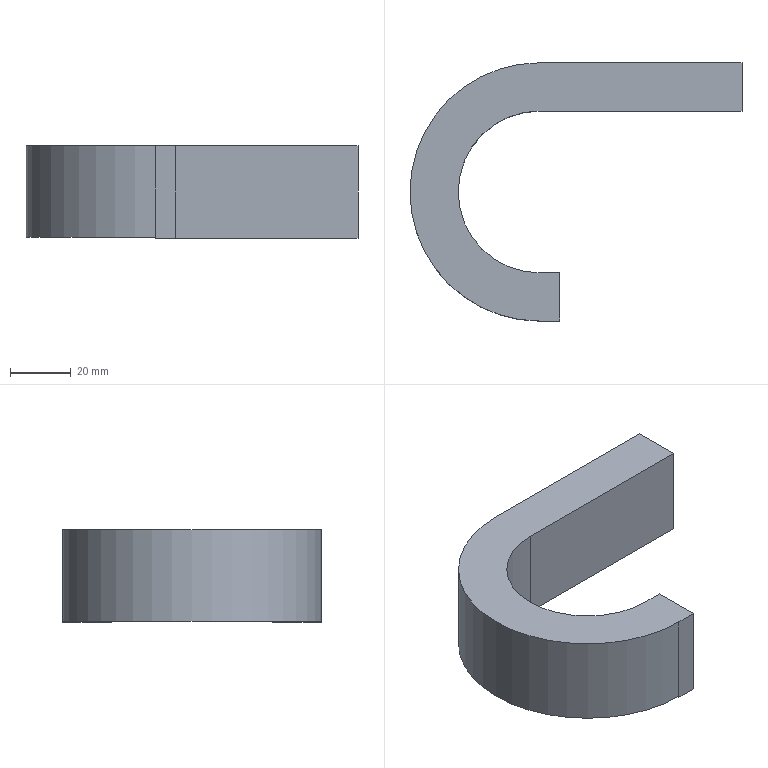Part | STEP file | RS40-AS-2LSR-T-266L-JR-Part-181 | 1 solid | 14 faces | box 109.3 x 85 x 30.35 mm | volume 87244 mm3 | plane 12 | cylinder 2 | commonest cylinder face diameters 53.238 x1 85 x1
STEP:
#1=CARTESIAN_POINT('',(1463.84,85.,30.35));
#2=VERTEX_POINT('',#1);
#3=CARTESIAN_POINT('',(1530.64,85.,30.35));
#4=VERTEX_POINT('',#3);
#5=CARTESIAN_POINT('',(1497.24,85.,30.35));
#6=DIRECTION('',(1.,0.,0.));
#7=VECTOR('',#6,1000.);
#8=LINE('',#5,#7);
#9=EDGE_CURVE('',#2,#4,#8,.T.);
#10=ORIENTED_EDGE('',*,*,#9,.F.);
#11=CARTESIAN_POINT('',(1463.84,0.00006,30.35));
#12=VERTEX_POINT('',#11);
#13=CARTESIAN_POINT('',(1463.84,42.5,30.35));
#14=DIRECTION('',(0.,0.,-1.));
#15=DIRECTION('',(0.,1.,0.));
#16=AXIS2_PLACEMENT_3D('',#13,#14,#15);
#17=CIRCLE('',#16,42.5);
#18=EDGE_CURVE('',#12,#2,#17,.T.);
#19=ORIENTED_EDGE('',*,*,#18,.F.);
#20=CARTESIAN_POINT('',(1470.64,0.00006,30.35));
#21=VERTEX_POINT('',#20);
#22=CARTESIAN_POINT('',(1467.24,0.00006,30.35));
#23=DIRECTION('',(-1.,0.,0.));
#24=VECTOR('',#23,1000.);
#25=LINE('',#22,#24);
#26=EDGE_CURVE('',#21,#12,#25,.T.);
#27=ORIENTED_EDGE('',*,*,#26,.F.);
#28=CARTESIAN_POINT('',(1470.64,15.881,30.35));
#29=VERTEX_POINT('',#28);
#30=CARTESIAN_POINT('',(1470.64,7.941,30.35));
#31=DIRECTION('',(0.,-1.,0.));
#32=VECTOR('',#31,1000.);
#33=LINE('',#30,#32);
#34=EDGE_CURVE('',#29,#21,#33,.T.);
#35=ORIENTED_EDGE('',*,*,#34,.F.);
#36=CARTESIAN_POINT('',(1463.84,15.881,30.35));
#37=VERTEX_POINT('',#36);
#38=CARTESIAN_POINT('',(1467.24,15.881,30.35));
#39=DIRECTION('',(1.,0.,0.));
#40=VECTOR('',#39,1000.);
#41=LINE('',#38,#40);
#42=EDGE_CURVE('',#37,#29,#41,.T.);
#43=ORIENTED_EDGE('',*,*,#42,.F.);
#44=CARTESIAN_POINT('',(1463.84,69.119,30.35));
#45=VERTEX_POINT('',#44);
#46=CARTESIAN_POINT('',(1463.84,42.5,30.35));
#47=DIRECTION('',(0.,0.,-1.));
#48=DIRECTION('',(0.,1.,0.));
#49=AXIS2_PLACEMENT_3D('',#46,#47,#48);
#50=CIRCLE('',#49,26.619);
#51=EDGE_CURVE('',#37,#45,#50,.T.);
#52=ORIENTED_EDGE('',*,*,#51,.T.);
#53=CARTESIAN_POINT('',(1530.64,69.119,30.35));
#54=VERTEX_POINT('',#53);
#55=CARTESIAN_POINT('',(1497.24,69.119,30.35));
#56=DIRECTION('',(-1.,0.,0.));
#57=VECTOR('',#56,1000.);
#58=LINE('',#55,#57);
#59=EDGE_CURVE('',#54,#45,#58,.T.);
#60=ORIENTED_EDGE('',*,*,#59,.F.);
#61=CARTESIAN_POINT('',(1530.64,77.06,30.35));
#62=DIRECTION('',(0.,-1.,0.));
#63=VECTOR('',#62,1000.);
#64=LINE('',#61,#63);
#65=EDGE_CURVE('',#4,#54,#64,.T.);
#66=ORIENTED_EDGE('',*,*,#65,.F.);
#67=EDGE_LOOP('',(#10,#19,#27,#35,#43,#52,#60,#66));
#68=FACE_OUTER_BOUND('',#67,.T.);
#69=CARTESIAN_POINT('',(1497.24,77.06,30.35));
#70=DIRECTION('',(0.,0.,1.));
#71=DIRECTION('',(0.,-1.,0.));
#72=AXIS2_PLACEMENT_3D('',#69,#70,#71);
#73=PLANE('',#72);
#74=ADVANCED_FACE('',(#68),#73,.T.);
#75=CARTESIAN_POINT('',(1463.84,85.,0.3249));
#76=VERTEX_POINT('',#75);
#77=CARTESIAN_POINT('',(1463.84,69.119,0.3249));
#78=VERTEX_POINT('',#77);
#79=CARTESIAN_POINT('',(1463.84,69.99,0.3249));
#80=DIRECTION('',(0.,-1.,0.));
#81=VECTOR('',#80,1000.);
#82=LINE('',#79,#81);
#83=EDGE_CURVE('',#76,#78,#82,.T.);
#84=ORIENTED_EDGE('',*,*,#83,.F.);
#85=CARTESIAN_POINT('',(1463.84,85.,0.));
#86=VERTEX_POINT('',#85);
#87=CARTESIAN_POINT('',(1463.84,85.,0.));
#88=DIRECTION('',(0.,0.,1.));
#89=VECTOR('',#88,1000.);
#90=LINE('',#87,#89);
#91=EDGE_CURVE('',#86,#76,#90,.T.);
#92=ORIENTED_EDGE('',*,*,#91,.F.);
#93=CARTESIAN_POINT('',(1463.84,69.119,0.));
#94=VERTEX_POINT('',#93);
#95=CARTESIAN_POINT('',(1463.84,77.06,0.));
#96=DIRECTION('',(0.,-1.,0.));
#97=VECTOR('',#96,1000.);
#98=LINE('',#95,#97);
#99=EDGE_CURVE('',#86,#94,#98,.T.);
#100=ORIENTED_EDGE('',*,*,#99,.T.);
#101=CARTESIAN_POINT('',(1463.84,69.119,0.));
#102=DIRECTION('',(0.,0.,1.));
#103=VECTOR('',#102,1000.);
#104=LINE('',#101,#103);
#105=EDGE_CURVE('',#94,#78,#104,.T.);
#106=ORIENTED_EDGE('',*,*,#105,.T.);
#107=EDGE_LOOP('',(#84,#92,#100,#106));
#108=FACE_OUTER_BOUND('',#107,.T.);
#109=CARTESIAN_POINT('',(1463.84,77.06,0.));
#110=DIRECTION('',(-1.,0.,0.));
#111=DIRECTION('',(0.,0.,-1.));
#112=AXIS2_PLACEMENT_3D('',#109,#110,#111);
#113=PLANE('',#112);
#114=ADVANCED_FACE('',(#108),#113,.T.);
#115=ORIENTED_EDGE('',*,*,#91,.T.);
#116=CARTESIAN_POINT('',(1463.84,85.,0.3249));
#117=DIRECTION('',(0.,0.,1.));
#118=VECTOR('',#117,1000.);
#119=LINE('',#116,#118);
#120=EDGE_CURVE('',#76,#2,#119,.T.);
#121=ORIENTED_EDGE('',*,*,#120,.T.);
#122=ORIENTED_EDGE('',*,*,#9,.T.);
#123=CARTESIAN_POINT('',(1530.64,85.,0.));
#124=VERTEX_POINT('',#123);
#125=CARTESIAN_POINT('',(1530.64,85.,0.));
#126=DIRECTION('',(0.,0.,1.));
#127=VECTOR('',#126,1000.);
#128=LINE('',#125,#127);
#129=EDGE_CURVE('',#124,#4,#128,.T.);
#130=ORIENTED_EDGE('',*,*,#129,.F.);
#131=CARTESIAN_POINT('',(1497.24,85.,0.));
#132=DIRECTION('',(-1.,0.,0.));
#133=VECTOR('',#132,1000.);
#134=LINE('',#131,#133);
#135=EDGE_CURVE('',#124,#86,#134,.T.);
#136=ORIENTED_EDGE('',*,*,#135,.T.);
#137=EDGE_LOOP('',(#115,#121,#122,#130,#136));
#138=FACE_OUTER_BOUND('',#137,.T.);
#139=CARTESIAN_POINT('',(1497.24,85.,0.));
#140=DIRECTION('',(0.,1.,0.));
#141=DIRECTION('',(0.,0.,1.));
#142=AXIS2_PLACEMENT_3D('',#139,#140,#141);
#143=PLANE('',#142);
#144=ADVANCED_FACE('',(#138),#143,.T.);
#145=ORIENTED_EDGE('',*,*,#129,.T.);
#146=ORIENTED_EDGE('',*,*,#65,.T.);
#147=CARTESIAN_POINT('',(1530.64,69.119,0.));
#148=VERTEX_POINT('',#147);
#149=CARTESIAN_POINT('',(1530.64,69.119,0.));
#150=DIRECTION('',(0.,0.,1.));
#151=VECTOR('',#150,1000.);
#152=LINE('',#149,#151);
#153=EDGE_CURVE('',#148,#54,#152,.T.);
#154=ORIENTED_EDGE('',*,*,#153,.F.);
#155=CARTESIAN_POINT('',(1530.64,77.06,0.));
#156=DIRECTION('',(0.,1.,0.));
#157=VECTOR('',#156,1000.);
#158=LINE('',#155,#157);
#159=EDGE_CURVE('',#148,#124,#158,.T.);
#160=ORIENTED_EDGE('',*,*,#159,.T.);
#161=EDGE_LOOP('',(#145,#146,#154,#160));
#162=FACE_OUTER_BOUND('',#161,.T.);
#163=CARTESIAN_POINT('',(1530.64,77.06,0.));
#164=DIRECTION('',(1.,0.,0.));
#165=DIRECTION('',(0.,0.,1.));
#166=AXIS2_PLACEMENT_3D('',#163,#164,#165);
#167=PLANE('',#166);
#168=ADVANCED_FACE('',(#162),#167,.T.);
#169=CARTESIAN_POINT('',(1497.24,69.119,0.));
#170=DIRECTION('',(1.,0.,0.));
#171=VECTOR('',#170,1000.);
#172=LINE('',#169,#171);
#173=EDGE_CURVE('',#94,#148,#172,.T.);
#174=ORIENTED_EDGE('',*,*,#173,.F.);
#175=ORIENTED_EDGE('',*,*,#99,.F.);
#176=ORIENTED_EDGE('',*,*,#135,.F.);
#177=ORIENTED_EDGE('',*,*,#159,.F.);
#178=EDGE_LOOP('',(#174,#175,#176,#177));
#179=FACE_OUTER_BOUND('',#178,.T.);
#180=CARTESIAN_POINT('',(1497.24,77.06,0.));
#181=DIRECTION('',(0.,0.,-1.));
#182=DIRECTION('',(0.,1.,0.));
#183=AXIS2_PLACEMENT_3D('',#180,#181,#182);
#184=PLANE('',#183);
#185=ADVANCED_FACE('',(#179),#184,.T.);
#186=ORIENTED_EDGE('',*,*,#173,.T.);
#187=ORIENTED_EDGE('',*,*,#153,.T.);
#188=ORIENTED_EDGE('',*,*,#59,.T.);
#189=CARTESIAN_POINT('',(1463.84,69.119,0.3249));
#190=DIRECTION('',(0.,0.,1.));
#191=VECTOR('',#190,1000.);
#192=LINE('',#189,#191);
#193=EDGE_CURVE('',#78,#45,#192,.T.);
#194=ORIENTED_EDGE('',*,*,#193,.F.);
#195=ORIENTED_EDGE('',*,*,#105,.F.);
#196=EDGE_LOOP('',(#186,#187,#188,#194,#195));
#197=FACE_OUTER_BOUND('',#196,.T.);
#198=CARTESIAN_POINT('',(1497.24,69.119,0.));
#199=DIRECTION('',(0.,-1.,0.));
#200=DIRECTION('',(0.,0.,-1.));
#201=AXIS2_PLACEMENT_3D('',#198,#199,#200);
#202=PLANE('',#201);
#203=ADVANCED_FACE('',(#197),#202,.T.);
#204=CARTESIAN_POINT('',(1463.84,15.881,0.3249));
#205=VERTEX_POINT('',#204);
#206=CARTESIAN_POINT('',(1463.84,0.00006,0.3249));
#207=VERTEX_POINT('',#206);
#208=CARTESIAN_POINT('',(1463.84,69.99,0.3249));
#209=DIRECTION('',(0.,-1.,0.));
#210=VECTOR('',#209,1000.);
#211=LINE('',#208,#210);
#212=EDGE_CURVE('',#205,#207,#211,.T.);
#213=ORIENTED_EDGE('',*,*,#212,.F.);
#214=CARTESIAN_POINT('',(1463.84,15.881,0.));
#215=VERTEX_POINT('',#214);
#216=CARTESIAN_POINT('',(1463.84,15.881,0.));
#217=DIRECTION('',(0.,0.,1.));
#218=VECTOR('',#217,1000.);
#219=LINE('',#216,#218);
#220=EDGE_CURVE('',#215,#205,#219,.T.);
#221=ORIENTED_EDGE('',*,*,#220,.F.);
#222=CARTESIAN_POINT('',(1463.84,0.00006,0.));
#223=VERTEX_POINT('',#222);
#224=CARTESIAN_POINT('',(1463.84,7.941,0.));
#225=DIRECTION('',(0.,-1.,0.));
#226=VECTOR('',#225,1000.);
#227=LINE('',#224,#226);
#228=EDGE_CURVE('',#215,#223,#227,.T.);
#229=ORIENTED_EDGE('',*,*,#228,.T.);
#230=CARTESIAN_POINT('',(1463.84,0.00006,0.));
#231=DIRECTION('',(0.,0.,1.));
#232=VECTOR('',#231,1000.);
#233=LINE('',#230,#232);
#234=EDGE_CURVE('',#223,#207,#233,.T.);
#235=ORIENTED_EDGE('',*,*,#234,.T.);
#236=EDGE_LOOP('',(#213,#221,#229,#235));
#237=FACE_OUTER_BOUND('',#236,.T.);
#238=CARTESIAN_POINT('',(1463.84,7.941,0.));
#239=DIRECTION('',(-1.,0.,0.));
#240=DIRECTION('',(0.,0.,-1.));
#241=AXIS2_PLACEMENT_3D('',#238,#239,#240);
#242=PLANE('',#241);
#243=ADVANCED_FACE('',(#237),#242,.T.);
#244=ORIENTED_EDGE('',*,*,#220,.T.);
#245=CARTESIAN_POINT('',(1463.84,15.881,0.3249));
#246=DIRECTION('',(0.,0.,-1.));
#247=VECTOR('',#246,1000.);
#248=LINE('',#245,#247);
#249=EDGE_CURVE('',#37,#205,#248,.T.);
#250=ORIENTED_EDGE('',*,*,#249,.F.);
#251=ORIENTED_EDGE('',*,*,#42,.T.);
#252=CARTESIAN_POINT('',(1470.64,15.881,0.));
#253=VERTEX_POINT('',#252);
#254=CARTESIAN_POINT('',(1470.64,15.881,0.));
#255=DIRECTION('',(0.,0.,1.));
#256=VECTOR('',#255,1000.);
#257=LINE('',#254,#256);
#258=EDGE_CURVE('',#253,#29,#257,.T.);
#259=ORIENTED_EDGE('',*,*,#258,.F.);
#260=CARTESIAN_POINT('',(1467.24,15.881,0.));
#261=DIRECTION('',(-1.,0.,0.));
#262=VECTOR('',#261,1000.);
#263=LINE('',#260,#262);
#264=EDGE_CURVE('',#253,#215,#263,.T.);
#265=ORIENTED_EDGE('',*,*,#264,.T.);
#266=EDGE_LOOP('',(#244,#250,#251,#259,#265));
#267=FACE_OUTER_BOUND('',#266,.T.);
#268=CARTESIAN_POINT('',(1467.24,15.881,0.));
#269=DIRECTION('',(0.,1.,0.));
#270=DIRECTION('',(0.,0.,1.));
#271=AXIS2_PLACEMENT_3D('',#268,#269,#270);
#272=PLANE('',#271);
#273=ADVANCED_FACE('',(#267),#272,.T.);
#274=ORIENTED_EDGE('',*,*,#258,.T.);
#275=ORIENTED_EDGE('',*,*,#34,.T.);
#276=CARTESIAN_POINT('',(1470.64,0.00006,0.));
#277=VERTEX_POINT('',#276);
#278=CARTESIAN_POINT('',(1470.64,0.00006,0.));
#279=DIRECTION('',(0.,0.,1.));
#280=VECTOR('',#279,1000.);
#281=LINE('',#278,#280);
#282=EDGE_CURVE('',#277,#21,#281,.T.);
#283=ORIENTED_EDGE('',*,*,#282,.F.);
#284=CARTESIAN_POINT('',(1470.64,7.941,0.));
#285=DIRECTION('',(0.,1.,0.));
#286=VECTOR('',#285,1000.);
#287=LINE('',#284,#286);
#288=EDGE_CURVE('',#277,#253,#287,.T.);
#289=ORIENTED_EDGE('',*,*,#288,.T.);
#290=EDGE_LOOP('',(#274,#275,#283,#289));
#291=FACE_OUTER_BOUND('',#290,.T.);
#292=CARTESIAN_POINT('',(1470.64,7.941,0.));
#293=DIRECTION('',(1.,0.,0.));
#294=DIRECTION('',(0.,0.,1.));
#295=AXIS2_PLACEMENT_3D('',#292,#293,#294);
#296=PLANE('',#295);
#297=ADVANCED_FACE('',(#291),#296,.T.);
#298=CARTESIAN_POINT('',(1467.24,0.00006,0.));
#299=DIRECTION('',(1.,0.,0.));
#300=VECTOR('',#299,1000.);
#301=LINE('',#298,#300);
#302=EDGE_CURVE('',#223,#277,#301,.T.);
#303=ORIENTED_EDGE('',*,*,#302,.F.);
#304=ORIENTED_EDGE('',*,*,#228,.F.);
#305=ORIENTED_EDGE('',*,*,#264,.F.);
#306=ORIENTED_EDGE('',*,*,#288,.F.);
#307=EDGE_LOOP('',(#303,#304,#305,#306));
#308=FACE_OUTER_BOUND('',#307,.T.);
#309=CARTESIAN_POINT('',(1467.24,7.941,0.));
#310=DIRECTION('',(0.,0.,-1.));
#311=DIRECTION('',(0.,1.,0.));
#312=AXIS2_PLACEMENT_3D('',#309,#310,#311);
#313=PLANE('',#312);
#314=ADVANCED_FACE('',(#308),#313,.T.);
#315=ORIENTED_EDGE('',*,*,#302,.T.);
#316=ORIENTED_EDGE('',*,*,#282,.T.);
#317=ORIENTED_EDGE('',*,*,#26,.T.);
#318=CARTESIAN_POINT('',(1463.84,0.00006,0.3249));
#319=DIRECTION('',(0.,0.,-1.));
#320=VECTOR('',#319,1000.);
#321=LINE('',#318,#320);
#322=EDGE_CURVE('',#12,#207,#321,.T.);
#323=ORIENTED_EDGE('',*,*,#322,.T.);
#324=ORIENTED_EDGE('',*,*,#234,.F.);
#325=EDGE_LOOP('',(#315,#316,#317,#323,#324));
#326=FACE_OUTER_BOUND('',#325,.T.);
#327=CARTESIAN_POINT('',(1467.24,0.00006,0.));
#328=DIRECTION('',(0.,-1.,0.));
#329=DIRECTION('',(0.,0.,-1.));
#330=AXIS2_PLACEMENT_3D('',#327,#328,#329);
#331=PLANE('',#330);
#332=ADVANCED_FACE('',(#326),#331,.T.);
#333=CARTESIAN_POINT('',(1463.84,42.5,0.3249));
#334=DIRECTION('',(0.,0.,1.));
#335=DIRECTION('',(0.,-1.,0.));
#336=AXIS2_PLACEMENT_3D('',#333,#334,#335);
#337=CIRCLE('',#336,42.5);
#338=EDGE_CURVE('',#76,#207,#337,.T.);
#339=ORIENTED_EDGE('',*,*,#338,.F.);
#340=ORIENTED_EDGE('',*,*,#83,.T.);
#341=CARTESIAN_POINT('',(1463.84,42.5,0.3249));
#342=DIRECTION('',(0.,0.,1.));
#343=DIRECTION('',(0.,-1.,0.));
#344=AXIS2_PLACEMENT_3D('',#341,#342,#343);
#345=CIRCLE('',#344,26.619);
#346=EDGE_CURVE('',#78,#205,#345,.T.);
#347=ORIENTED_EDGE('',*,*,#346,.T.);
#348=ORIENTED_EDGE('',*,*,#212,.T.);
#349=EDGE_LOOP('',(#339,#340,#347,#348));
#350=FACE_OUTER_BOUND('',#349,.T.);
#351=CARTESIAN_POINT('',(1463.84,42.5,0.3249));
#352=DIRECTION('',(0.,0.,-1.));
#353=DIRECTION('',(0.,1.,0.));
#354=AXIS2_PLACEMENT_3D('',#351,#352,#353);
#355=PLANE('',#354);
#356=ADVANCED_FACE('',(#350),#355,.T.);
#357=ORIENTED_EDGE('',*,*,#322,.F.);
#358=ORIENTED_EDGE('',*,*,#18,.T.);
#359=ORIENTED_EDGE('',*,*,#120,.F.);
#360=ORIENTED_EDGE('',*,*,#338,.T.);
#361=EDGE_LOOP('',(#357,#358,#359,#360));
#362=FACE_OUTER_BOUND('',#361,.T.);
#363=CARTESIAN_POINT('',(1463.84,42.5,0.3249));
#364=DIRECTION('',(0.,0.,1.));
#365=DIRECTION('',(0.,-1.,0.));
#366=AXIS2_PLACEMENT_3D('',#363,#364,#365);
#367=CYLINDRICAL_SURFACE('',#366,42.5);
#368=ADVANCED_FACE('',(#362),#367,.T.);
#369=ORIENTED_EDGE('',*,*,#51,.F.);
#370=ORIENTED_EDGE('',*,*,#249,.T.);
#371=ORIENTED_EDGE('',*,*,#346,.F.);
#372=ORIENTED_EDGE('',*,*,#193,.T.);
#373=EDGE_LOOP('',(#369,#370,#371,#372));
#374=FACE_OUTER_BOUND('',#373,.T.);
#375=CARTESIAN_POINT('',(1463.84,42.5,0.3249));
#376=DIRECTION('',(0.,0.,1.));
#377=DIRECTION('',(0.,-1.,0.));
#378=AXIS2_PLACEMENT_3D('',#375,#376,#377);
#379=CYLINDRICAL_SURFACE('',#378,26.619);
#380=ADVANCED_FACE('',(#374),#379,.F.);
#381=CLOSED_SHELL('',(#74,#114,#144,#168,#185,#203,#243,#273,#297,#314,#332,#356,#368,#380));
#382=MANIFOLD_SOLID_BREP('',#381);
#383=CARTESIAN_POINT('',(0.,0.,0.));
#384=DIRECTION('',(0.,0.,1.));
#385=DIRECTION('',(1.,0.,0.));
#386=AXIS2_PLACEMENT_3D('',#383,#384,#385);
#387=(LENGTH_UNIT()NAMED_UNIT(*)SI_UNIT(.MILLI.,.METRE.));
#388=UNCERTAINTY_MEASURE_WITH_UNIT(LENGTH_MEASURE(0.00001),#387,'','');
#389=(NAMED_UNIT(*)PLANE_ANGLE_UNIT()SI_UNIT($,.RADIAN.));
#390=(NAMED_UNIT(*)SI_UNIT($,.STERADIAN.)SOLID_ANGLE_UNIT());
#391=(GEOMETRIC_REPRESENTATION_CONTEXT(3)GLOBAL_UNCERTAINTY_ASSIGNED_CONTEXT((#388))GLOBAL_UNIT_ASSIGNED_CONTEXT((#387,#389,#390))REPRESENTATION_CONTEXT('',''));
#392=ADVANCED_BREP_SHAPE_REPRESENTATION('',(#382,#386),#391);